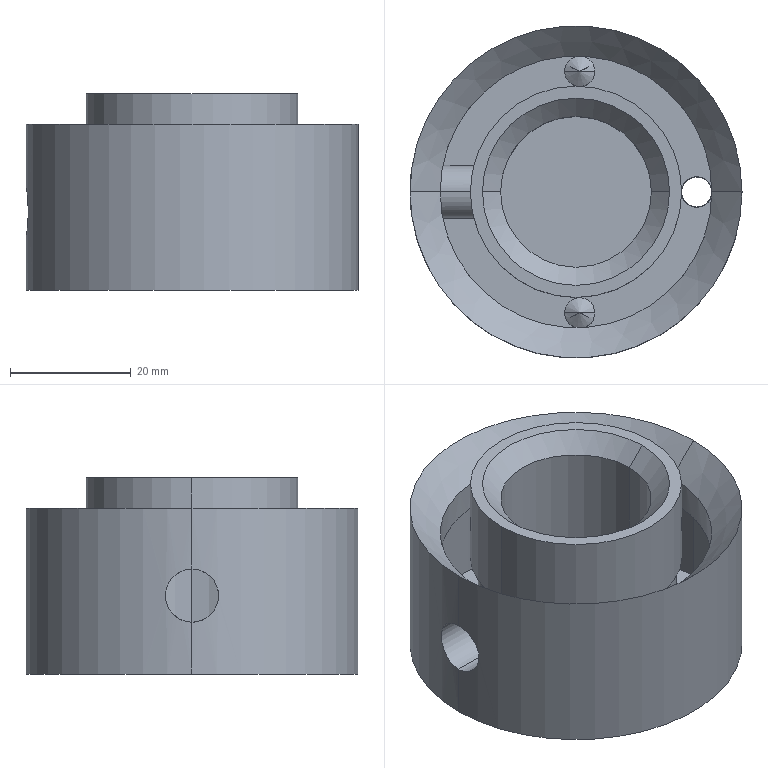Part | 1 solid | 28 faces | box 55 x 55 x 32.5 mm | volume 47312 mm3 | cylinder 16 | cone 8 | plane 4 | commonest cylinder face diameters 5 x6 8.8 x2 25 x2 35 x2 45 x2 55 x2
STEP:
#1=CARTESIAN_POINT('',(-12.5,0.,29.5));
#2=VERTEX_POINT('',#1);
#3=CARTESIAN_POINT('',(12.5,0.,29.5));
#4=VERTEX_POINT('',#3);
#5=CARTESIAN_POINT('',(0.,0.,29.5));
#6=DIRECTION('',(0.,0.,1.));
#7=DIRECTION('',(1.,0.,0.));
#8=AXIS2_PLACEMENT_3D('',#5,#6,#7);
#9=CIRCLE('',#8,12.5);
#10=EDGE_CURVE('',#2,#4,#9,.T.);
#11=ORIENTED_EDGE('',*,*,#10,.F.);
#12=CARTESIAN_POINT('',(-15.5,0.,32.5));
#13=VERTEX_POINT('',#12);
#14=CARTESIAN_POINT('',(-12.5,0.,29.5));
#15=DIRECTION('',(-0.7071,0.,0.7071));
#16=VECTOR('',#15,1000.);
#17=LINE('',#14,#16);
#18=EDGE_CURVE('',#2,#13,#17,.T.);
#19=ORIENTED_EDGE('',*,*,#18,.T.);
#20=CARTESIAN_POINT('',(15.5,0.,32.5));
#21=VERTEX_POINT('',#20);
#22=CARTESIAN_POINT('',(0.,0.,32.5));
#23=DIRECTION('',(0.,0.,-1.));
#24=DIRECTION('',(1.,0.,0.));
#25=AXIS2_PLACEMENT_3D('',#22,#23,#24);
#26=CIRCLE('',#25,15.5);
#27=EDGE_CURVE('',#21,#13,#26,.T.);
#28=ORIENTED_EDGE('',*,*,#27,.F.);
#29=CARTESIAN_POINT('',(12.5,0.,29.5));
#30=DIRECTION('',(0.7071,0.,0.7071));
#31=VECTOR('',#30,1000.);
#32=LINE('',#29,#31);
#33=EDGE_CURVE('',#4,#21,#32,.T.);
#34=ORIENTED_EDGE('',*,*,#33,.F.);
#35=EDGE_LOOP('',(#11,#19,#28,#34));
#36=FACE_OUTER_BOUND('',#35,.T.);
#37=CARTESIAN_POINT('',(0.,0.,29.5));
#38=DIRECTION('',(0.,0.,1.));
#39=DIRECTION('',(1.,0.,0.));
#40=AXIS2_PLACEMENT_3D('',#37,#38,#39);
#41=CONICAL_SURFACE('',#40,12.5,0.7854);
#42=ADVANCED_FACE('',(#36),#41,.F.);
#43=CARTESIAN_POINT('',(17.5,0.,0.));
#44=VERTEX_POINT('',#43);
#45=CARTESIAN_POINT('',(22.5,0.,0.));
#46=VERTEX_POINT('',#45);
#47=CARTESIAN_POINT('',(20.,0.,0.));
#48=DIRECTION('',(0.,0.,1.));
#49=DIRECTION('',(1.,0.,0.));
#50=AXIS2_PLACEMENT_3D('',#47,#48,#49);
#51=CIRCLE('',#50,2.5);
#52=EDGE_CURVE('',#44,#46,#51,.T.);
#53=ORIENTED_EDGE('',*,*,#52,.F.);
#54=CARTESIAN_POINT('',(17.5,0.,17.5));
#55=VERTEX_POINT('',#54);
#56=CARTESIAN_POINT('',(17.5,0.,17.5));
#57=DIRECTION('',(0.,0.,1.));
#58=VECTOR('',#57,1000.);
#59=LINE('',#56,#58);
#60=EDGE_CURVE('',#44,#55,#59,.T.);
#61=ORIENTED_EDGE('',*,*,#60,.T.);
#62=CARTESIAN_POINT('',(22.5,0.,17.5));
#63=VERTEX_POINT('',#62);
#64=CARTESIAN_POINT('',(20.,0.,17.5));
#65=DIRECTION('',(0.,0.,1.));
#66=DIRECTION('',(1.,0.,0.));
#67=AXIS2_PLACEMENT_3D('',#64,#65,#66);
#68=CIRCLE('',#67,2.5);
#69=EDGE_CURVE('',#55,#63,#68,.T.);
#70=ORIENTED_EDGE('',*,*,#69,.T.);
#71=CARTESIAN_POINT('',(22.5,0.,17.5));
#72=DIRECTION('',(0.,0.,1.));
#73=VECTOR('',#72,1000.);
#74=LINE('',#71,#73);
#75=EDGE_CURVE('',#46,#63,#74,.T.);
#76=ORIENTED_EDGE('',*,*,#75,.F.);
#77=EDGE_LOOP('',(#53,#61,#70,#76));
#78=FACE_OUTER_BOUND('',#77,.T.);
#79=CARTESIAN_POINT('',(20.,0.,17.5));
#80=DIRECTION('',(0.,0.,1.));
#81=DIRECTION('',(1.,0.,0.));
#82=AXIS2_PLACEMENT_3D('',#79,#80,#81);
#83=CYLINDRICAL_SURFACE('',#82,2.5);
#84=ADVANCED_FACE('',(#78),#83,.F.);
#85=CARTESIAN_POINT('',(-27.5,0.,17.4));
#86=VERTEX_POINT('',#85);
#87=CARTESIAN_POINT('',(-27.5,0.,8.6));
#88=VERTEX_POINT('',#87);
#89=CARTESIAN_POINT('',(-27.5,0.,17.4));
#90=CARTESIAN_POINT('',(-27.5,-0.2873,17.4));
#91=CARTESIAN_POINT('',(-27.495,-0.5732,17.372));
#92=CARTESIAN_POINT('',(-27.478,-1.142,17.259));
#93=CARTESIAN_POINT('',(-27.465,-1.419,17.175));
#94=CARTESIAN_POINT('',(-27.432,-1.949,16.955));
#95=CARTESIAN_POINT('',(-27.412,-2.205,16.818));
#96=CARTESIAN_POINT('',(-27.37,-2.685,16.498));
#97=CARTESIAN_POINT('',(-27.347,-2.906,16.316));
#98=CARTESIAN_POINT('',(-27.301,-3.312,15.911));
#99=CARTESIAN_POINT('',(-27.277,-3.498,15.685));
#100=CARTESIAN_POINT('',(-27.234,-3.817,15.208));
#101=CARTESIAN_POINT('',(-27.215,-3.952,14.955));
#102=CARTESIAN_POINT('',(-27.182,-4.174,14.422));
#103=CARTESIAN_POINT('',(-27.168,-4.259,14.143));
#104=CARTESIAN_POINT('',(-27.15,-4.371,13.581));
#105=CARTESIAN_POINT('',(-27.146,-4.4,13.293));
#106=CARTESIAN_POINT('',(-27.146,-4.4,12.712));
#107=CARTESIAN_POINT('',(-27.15,-4.372,12.426));
#108=CARTESIAN_POINT('',(-27.168,-4.26,11.863));
#109=CARTESIAN_POINT('',(-27.181,-4.175,11.583));
#110=CARTESIAN_POINT('',(-27.214,-3.955,11.05));
#111=CARTESIAN_POINT('',(-27.234,-3.82,10.798));
#112=CARTESIAN_POINT('',(-27.277,-3.501,10.319));
#113=CARTESIAN_POINT('',(-27.3,-3.316,10.093));
#114=CARTESIAN_POINT('',(-27.346,-2.911,9.688));
#115=CARTESIAN_POINT('',(-27.369,-2.69,9.506));
#116=CARTESIAN_POINT('',(-27.412,-2.209,9.183));
#117=CARTESIAN_POINT('',(-27.432,-1.954,9.047));
#118=CARTESIAN_POINT('',(-27.464,-1.425,8.827));
#119=CARTESIAN_POINT('',(-27.478,-1.147,8.742));
#120=CARTESIAN_POINT('',(-27.495,-0.5788,8.629));
#121=CARTESIAN_POINT('',(-27.5,-0.2911,8.6));
#122=CARTESIAN_POINT('',(-27.5,0.,8.6));
#123=B_SPLINE_CURVE_WITH_KNOTS('',3,(#89,#90,#91,#92,#93,#94,#95,#96,#97,#98,#99,#100,#101,#102,#103,#104,#105,#106,#107,#108,#109,#110,#111,#112,#113,#114,#115,#116,#117,#118,#119,#120,#121,#122),.UNSPECIFIED.,.F.,.F.,(4,2,2,2,2,2,2,2,2,2,2,2,2,2,2,2,4),(0.01378,0.01464,0.0155,0.01636,0.01722,0.01808,0.01894,0.01981,0.02067,0.02153,0.02239,0.02325,0.02411,0.02497,0.02583,0.02669,0.02755),.UNSPECIFIED.);
#124=EDGE_CURVE('',#86,#88,#123,.T.);
#125=ORIENTED_EDGE('',*,*,#124,.F.);
#126=CARTESIAN_POINT('',(-12.5,0.,17.4));
#127=VERTEX_POINT('',#126);
#128=CARTESIAN_POINT('',(0.,0.,17.4));
#129=DIRECTION('',(1.,0.,0.));
#130=VECTOR('',#129,1000.);
#131=LINE('',#128,#130);
#132=EDGE_CURVE('',#86,#127,#131,.T.);
#133=ORIENTED_EDGE('',*,*,#132,.T.);
#134=CARTESIAN_POINT('',(-12.5,0.,8.6));
#135=VERTEX_POINT('',#134);
#136=CARTESIAN_POINT('',(-12.5,0.,17.4));
#137=CARTESIAN_POINT('',(-12.5,-0.2933,17.4));
#138=CARTESIAN_POINT('',(-12.49,-0.5812,17.371));
#139=CARTESIAN_POINT('',(-12.451,-1.147,17.258));
#140=CARTESIAN_POINT('',(-12.421,-1.428,17.172));
#141=CARTESIAN_POINT('',(-12.348,-1.96,16.95));
#142=CARTESIAN_POINT('',(-12.305,-2.211,16.815));
#143=CARTESIAN_POINT('',(-12.21,-2.688,16.495));
#144=CARTESIAN_POINT('',(-12.158,-2.912,16.311));
#145=CARTESIAN_POINT('',(-12.055,-3.314,15.908));
#146=CARTESIAN_POINT('',(-12.003,-3.495,15.688));
#147=CARTESIAN_POINT('',(-11.904,-3.817,15.208));
#148=CARTESIAN_POINT('',(-11.86,-3.952,14.956));
#149=CARTESIAN_POINT('',(-11.803,-4.117,14.56));
#150=CARTESIAN_POINT('',(-11.786,-4.165,14.425));
#151=CARTESIAN_POINT('',(-11.755,-4.25,14.148));
#152=CARTESIAN_POINT('',(-11.742,-4.286,14.006));
#153=CARTESIAN_POINT('',(-11.711,-4.371,13.579));
#154=CARTESIAN_POINT('',(-11.7,-4.4,13.292));
#155=CARTESIAN_POINT('',(-11.7,-4.4,12.713));
#156=CARTESIAN_POINT('',(-11.711,-4.371,12.418));
#157=CARTESIAN_POINT('',(-11.753,-4.257,11.852));
#158=CARTESIAN_POINT('',(-11.783,-4.173,11.577));
#159=CARTESIAN_POINT('',(-11.86,-3.95,11.041));
#160=CARTESIAN_POINT('',(-11.905,-3.814,10.788));
#161=CARTESIAN_POINT('',(-12.002,-3.496,10.314));
#162=CARTESIAN_POINT('',(-12.055,-3.312,10.09));
#163=CARTESIAN_POINT('',(-12.159,-2.908,9.685));
#164=CARTESIAN_POINT('',(-12.21,-2.688,9.505));
#165=CARTESIAN_POINT('',(-12.305,-2.213,9.186));
#166=CARTESIAN_POINT('',(-12.349,-1.955,9.048));
#167=CARTESIAN_POINT('',(-12.421,-1.426,8.828));
#168=CARTESIAN_POINT('',(-12.45,-1.151,8.743));
#169=CARTESIAN_POINT('',(-12.49,-0.5803,8.629));
#170=CARTESIAN_POINT('',(-12.5,-0.2889,8.6));
#171=CARTESIAN_POINT('',(-12.5,0.,8.6));
#172=B_SPLINE_CURVE_WITH_KNOTS('',3,(#136,#137,#138,#139,#140,#141,#142,#143,#144,#145,#146,#147,#148,#149,#150,#151,#152,#153,#154,#155,#156,#157,#158,#159,#160,#161,#162,#163,#164,#165,#166,#167,#168,#169,#170,#171),.UNSPECIFIED.,.F.,.F.,(4,2,2,2,2,2,2,2,2,2,2,2,2,2,2,2,2,4),(0.,0.0008668,0.001734,0.0026,0.003467,0.004334,0.005201,0.005634,0.006067,0.006934,0.007801,0.008668,0.009535,0.0104,0.01127,0.01213,0.013,0.01387),.UNSPECIFIED.);
#173=EDGE_CURVE('',#127,#135,#172,.T.);
#174=ORIENTED_EDGE('',*,*,#173,.T.);
#175=CARTESIAN_POINT('',(0.,0.,8.6));
#176=DIRECTION('',(1.,0.,0.));
#177=VECTOR('',#176,1000.);
#178=LINE('',#175,#177);
#179=EDGE_CURVE('',#88,#135,#178,.T.);
#180=ORIENTED_EDGE('',*,*,#179,.F.);
#181=EDGE_LOOP('',(#125,#133,#174,#180));
#182=FACE_OUTER_BOUND('',#181,.T.);
#183=CARTESIAN_POINT('',(0.,0.,13.));
#184=DIRECTION('',(1.,0.,0.));
#185=DIRECTION('',(0.,0.,-1.));
#186=AXIS2_PLACEMENT_3D('',#183,#184,#185);
#187=CYLINDRICAL_SURFACE('',#186,4.4);
#188=ADVANCED_FACE('',(#182),#187,.F.);
#189=CARTESIAN_POINT('',(3.117,19.99,12.));
#190=VERTEX_POINT('',#189);
#191=CARTESIAN_POINT('',(-1.883,19.99,12.));
#192=VERTEX_POINT('',#191);
#193=CARTESIAN_POINT('',(0.6172,19.99,12.));
#194=DIRECTION('',(0.,0.,-1.));
#195=DIRECTION('',(-1.,0.,0.));
#196=AXIS2_PLACEMENT_3D('',#193,#194,#195);
#197=CIRCLE('',#196,2.5);
#198=EDGE_CURVE('',#190,#192,#197,.T.);
#199=ORIENTED_EDGE('',*,*,#198,.F.);
#200=CARTESIAN_POINT('',(3.117,19.99,0.));
#201=VERTEX_POINT('',#200);
#202=CARTESIAN_POINT('',(3.117,19.99,0.));
#203=DIRECTION('',(0.,0.,-1.));
#204=VECTOR('',#203,1000.);
#205=LINE('',#202,#204);
#206=EDGE_CURVE('',#190,#201,#205,.T.);
#207=ORIENTED_EDGE('',*,*,#206,.T.);
#208=CARTESIAN_POINT('',(-1.883,19.99,0.));
#209=VERTEX_POINT('',#208);
#210=CARTESIAN_POINT('',(0.6172,19.99,0.));
#211=DIRECTION('',(0.,0.,-1.));
#212=DIRECTION('',(-1.,0.,0.));
#213=AXIS2_PLACEMENT_3D('',#210,#211,#212);
#214=CIRCLE('',#213,2.5);
#215=EDGE_CURVE('',#201,#209,#214,.T.);
#216=ORIENTED_EDGE('',*,*,#215,.T.);
#217=CARTESIAN_POINT('',(-1.883,19.99,0.));
#218=DIRECTION('',(0.,0.,-1.));
#219=VECTOR('',#218,1000.);
#220=LINE('',#217,#219);
#221=EDGE_CURVE('',#192,#209,#220,.T.);
#222=ORIENTED_EDGE('',*,*,#221,.F.);
#223=EDGE_LOOP('',(#199,#207,#216,#222));
#224=FACE_OUTER_BOUND('',#223,.T.);
#225=CARTESIAN_POINT('',(0.6172,19.99,0.));
#226=DIRECTION('',(0.,0.,-1.));
#227=DIRECTION('',(-1.,0.,0.));
#228=AXIS2_PLACEMENT_3D('',#225,#226,#227);
#229=CYLINDRICAL_SURFACE('',#228,2.5);
#230=ADVANCED_FACE('',(#224),#229,.F.);
#231=CARTESIAN_POINT('',(0.6172,19.99,13.502));
#232=VERTEX_POINT('',#231);
#233=CARTESIAN_POINT('',(-1.883,19.99,12.));
#234=DIRECTION('',(-0.8572,0.,-0.515));
#235=VECTOR('',#234,1000.);
#236=LINE('',#233,#235);
#237=EDGE_CURVE('',#232,#192,#236,.T.);
#238=ORIENTED_EDGE('',*,*,#237,.F.);
#239=CARTESIAN_POINT('',(3.117,19.99,12.));
#240=DIRECTION('',(0.8572,0.,-0.515));
#241=VECTOR('',#240,1000.);
#242=LINE('',#239,#241);
#243=EDGE_CURVE('',#232,#190,#242,.T.);
#244=ORIENTED_EDGE('',*,*,#243,.T.);
#245=ORIENTED_EDGE('',*,*,#198,.T.);
#246=EDGE_LOOP('',(#238,#244,#245));
#247=FACE_OUTER_BOUND('',#246,.T.);
#248=CARTESIAN_POINT('',(0.6172,19.99,12.));
#249=DIRECTION('',(0.,0.,-1.));
#250=DIRECTION('',(-1.,0.,0.));
#251=AXIS2_PLACEMENT_3D('',#248,#249,#250);
#252=CONICAL_SURFACE('',#251,2.5,1.03);
#253=ADVANCED_FACE('',(#247),#252,.F.);
#254=CARTESIAN_POINT('',(3.12,-20.028,12.));
#255=VERTEX_POINT('',#254);
#256=CARTESIAN_POINT('',(-1.88,-20.028,12.));
#257=VERTEX_POINT('',#256);
#258=CARTESIAN_POINT('',(0.6196,-20.028,12.));
#259=DIRECTION('',(0.,0.,-1.));
#260=DIRECTION('',(-1.,0.,0.));
#261=AXIS2_PLACEMENT_3D('',#258,#259,#260);
#262=CIRCLE('',#261,2.5);
#263=EDGE_CURVE('',#255,#257,#262,.T.);
#264=ORIENTED_EDGE('',*,*,#263,.F.);
#265=CARTESIAN_POINT('',(3.12,-20.028,0.));
#266=VERTEX_POINT('',#265);
#267=CARTESIAN_POINT('',(3.12,-20.028,0.));
#268=DIRECTION('',(0.,0.,-1.));
#269=VECTOR('',#268,1000.);
#270=LINE('',#267,#269);
#271=EDGE_CURVE('',#255,#266,#270,.T.);
#272=ORIENTED_EDGE('',*,*,#271,.T.);
#273=CARTESIAN_POINT('',(-1.88,-20.028,0.));
#274=VERTEX_POINT('',#273);
#275=CARTESIAN_POINT('',(0.6196,-20.028,0.));
#276=DIRECTION('',(0.,0.,-1.));
#277=DIRECTION('',(-1.,0.,0.));
#278=AXIS2_PLACEMENT_3D('',#275,#276,#277);
#279=CIRCLE('',#278,2.5);
#280=EDGE_CURVE('',#266,#274,#279,.T.);
#281=ORIENTED_EDGE('',*,*,#280,.T.);
#282=CARTESIAN_POINT('',(-1.88,-20.028,0.));
#283=DIRECTION('',(0.,0.,-1.));
#284=VECTOR('',#283,1000.);
#285=LINE('',#282,#284);
#286=EDGE_CURVE('',#257,#274,#285,.T.);
#287=ORIENTED_EDGE('',*,*,#286,.F.);
#288=EDGE_LOOP('',(#264,#272,#281,#287));
#289=FACE_OUTER_BOUND('',#288,.T.);
#290=CARTESIAN_POINT('',(0.6196,-20.028,0.));
#291=DIRECTION('',(0.,0.,-1.));
#292=DIRECTION('',(-1.,0.,0.));
#293=AXIS2_PLACEMENT_3D('',#290,#291,#292);
#294=CYLINDRICAL_SURFACE('',#293,2.5);
#295=ADVANCED_FACE('',(#289),#294,.F.);
#296=CARTESIAN_POINT('',(0.6196,-20.028,13.502));
#297=VERTEX_POINT('',#296);
#298=CARTESIAN_POINT('',(-1.88,-20.028,12.));
#299=DIRECTION('',(-0.8572,0.,-0.515));
#300=VECTOR('',#299,1000.);
#301=LINE('',#298,#300);
#302=EDGE_CURVE('',#297,#257,#301,.T.);
#303=ORIENTED_EDGE('',*,*,#302,.F.);
#304=CARTESIAN_POINT('',(3.12,-20.028,12.));
#305=DIRECTION('',(0.8572,0.,-0.515));
#306=VECTOR('',#305,1000.);
#307=LINE('',#304,#306);
#308=EDGE_CURVE('',#297,#255,#307,.T.);
#309=ORIENTED_EDGE('',*,*,#308,.T.);
#310=ORIENTED_EDGE('',*,*,#263,.T.);
#311=EDGE_LOOP('',(#303,#309,#310));
#312=FACE_OUTER_BOUND('',#311,.T.);
#313=CARTESIAN_POINT('',(0.6196,-20.028,12.));
#314=DIRECTION('',(0.,0.,-1.));
#315=DIRECTION('',(-1.,0.,0.));
#316=AXIS2_PLACEMENT_3D('',#313,#314,#315);
#317=CONICAL_SURFACE('',#316,2.5,1.03);
#318=ADVANCED_FACE('',(#312),#317,.F.);
#319=CARTESIAN_POINT('',(-22.5,0.,22.5));
#320=VERTEX_POINT('',#319);
#321=CARTESIAN_POINT('',(22.5,0.,22.5));
#322=VERTEX_POINT('',#321);
#323=CARTESIAN_POINT('',(0.,0.,22.5));
#324=DIRECTION('',(0.,0.,1.));
#325=DIRECTION('',(1.,0.,0.));
#326=AXIS2_PLACEMENT_3D('',#323,#324,#325);
#327=CIRCLE('',#326,22.5);
#328=EDGE_CURVE('',#320,#322,#327,.T.);
#329=ORIENTED_EDGE('',*,*,#328,.F.);
#330=CARTESIAN_POINT('',(-27.5,0.,27.5));
#331=VERTEX_POINT('',#330);
#332=CARTESIAN_POINT('',(-22.5,0.,22.5));
#333=DIRECTION('',(-0.7071,0.,0.7071));
#334=VECTOR('',#333,1000.);
#335=LINE('',#332,#334);
#336=EDGE_CURVE('',#320,#331,#335,.T.);
#337=ORIENTED_EDGE('',*,*,#336,.T.);
#338=CARTESIAN_POINT('',(27.5,0.,27.5));
#339=VERTEX_POINT('',#338);
#340=CARTESIAN_POINT('',(0.,0.,27.5));
#341=DIRECTION('',(0.,0.,1.));
#342=DIRECTION('',(1.,0.,0.));
#343=AXIS2_PLACEMENT_3D('',#340,#341,#342);
#344=CIRCLE('',#343,27.5);
#345=EDGE_CURVE('',#331,#339,#344,.T.);
#346=ORIENTED_EDGE('',*,*,#345,.T.);
#347=CARTESIAN_POINT('',(22.5,0.,22.5));
#348=DIRECTION('',(0.7071,0.,0.7071));
#349=VECTOR('',#348,1000.);
#350=LINE('',#347,#349);
#351=EDGE_CURVE('',#322,#339,#350,.T.);
#352=ORIENTED_EDGE('',*,*,#351,.F.);
#353=EDGE_LOOP('',(#329,#337,#346,#352));
#354=FACE_OUTER_BOUND('',#353,.T.);
#355=CARTESIAN_POINT('',(0.,0.,22.5));
#356=DIRECTION('',(0.,0.,1.));
#357=DIRECTION('',(1.,0.,0.));
#358=AXIS2_PLACEMENT_3D('',#355,#356,#357);
#359=CONICAL_SURFACE('',#358,22.5,0.7854);
#360=ADVANCED_FACE('',(#354),#359,.F.);
#361=CARTESIAN_POINT('',(0.,0.,27.5));
#362=DIRECTION('',(0.,0.,1.));
#363=DIRECTION('',(1.,0.,0.));
#364=AXIS2_PLACEMENT_3D('',#361,#362,#363);
#365=CIRCLE('',#364,27.5);
#366=EDGE_CURVE('',#339,#331,#365,.T.);
#367=ORIENTED_EDGE('',*,*,#366,.F.);
#368=CARTESIAN_POINT('',(27.5,0.,0.));
#369=VERTEX_POINT('',#368);
#370=CARTESIAN_POINT('',(27.5,0.,32.5));
#371=DIRECTION('',(0.,0.,-1.));
#372=VECTOR('',#371,1000.);
#373=LINE('',#370,#372);
#374=EDGE_CURVE('',#339,#369,#373,.T.);
#375=ORIENTED_EDGE('',*,*,#374,.T.);
#376=CARTESIAN_POINT('',(-27.5,0.,0.));
#377=VERTEX_POINT('',#376);
#378=CARTESIAN_POINT('',(0.,0.,0.));
#379=DIRECTION('',(0.,0.,1.));
#380=DIRECTION('',(1.,0.,0.));
#381=AXIS2_PLACEMENT_3D('',#378,#379,#380);
#382=CIRCLE('',#381,27.5);
#383=EDGE_CURVE('',#369,#377,#382,.T.);
#384=ORIENTED_EDGE('',*,*,#383,.T.);
#385=CARTESIAN_POINT('',(-27.5,0.,32.5));
#386=DIRECTION('',(0.,0.,-1.));
#387=VECTOR('',#386,1000.);
#388=LINE('',#385,#387);
#389=EDGE_CURVE('',#88,#377,#388,.T.);
#390=ORIENTED_EDGE('',*,*,#389,.F.);
#391=CARTESIAN_POINT('',(-27.5,0.,8.6));
#392=CARTESIAN_POINT('',(-27.5,0.2912,8.6));
#393=CARTESIAN_POINT('',(-27.495,0.5775,8.629));
#394=CARTESIAN_POINT('',(-27.478,1.141,8.741));
#395=CARTESIAN_POINT('',(-27.465,1.42,8.826));
#396=CARTESIAN_POINT('',(-27.432,1.953,9.047));
#397=CARTESIAN_POINT('',(-27.412,2.205,9.182));
#398=CARTESIAN_POINT('',(-27.37,2.683,9.501));
#399=CARTESIAN_POINT('',(-27.346,2.909,9.687));
#400=CARTESIAN_POINT('',(-27.3,3.315,10.092));
#401=CARTESIAN_POINT('',(-27.277,3.496,10.313));
#402=CARTESIAN_POINT('',(-27.234,3.818,10.794));
#403=CARTESIAN_POINT('',(-27.214,3.955,11.05));
#404=CARTESIAN_POINT('',(-27.182,4.174,11.579));
#405=CARTESIAN_POINT('',(-27.168,4.259,11.857));
#406=CARTESIAN_POINT('',(-27.15,4.372,12.425));
#407=CARTESIAN_POINT('',(-27.146,4.4,12.711));
#408=CARTESIAN_POINT('',(-27.146,4.4,13.286));
#409=CARTESIAN_POINT('',(-27.15,4.371,13.578));
#410=CARTESIAN_POINT('',(-27.168,4.259,14.143));
#411=CARTESIAN_POINT('',(-27.181,4.176,14.417));
#412=CARTESIAN_POINT('',(-27.214,3.955,14.95));
#413=CARTESIAN_POINT('',(-27.234,3.817,15.207));
#414=CARTESIAN_POINT('',(-27.277,3.499,15.684));
#415=CARTESIAN_POINT('',(-27.3,3.316,15.906));
#416=CARTESIAN_POINT('',(-27.347,2.906,16.316));
#417=CARTESIAN_POINT('',(-27.37,2.685,16.498));
#418=CARTESIAN_POINT('',(-27.412,2.209,16.816));
#419=CARTESIAN_POINT('',(-27.432,1.951,16.954));
#420=CARTESIAN_POINT('',(-27.465,1.419,17.175));
#421=CARTESIAN_POINT('',(-27.478,1.144,17.258));
#422=CARTESIAN_POINT('',(-27.495,0.5794,17.371));
#423=CARTESIAN_POINT('',(-27.5,0.2874,17.4));
#424=CARTESIAN_POINT('',(-27.5,0.,17.4));
#425=B_SPLINE_CURVE_WITH_KNOTS('',3,(#391,#392,#393,#394,#395,#396,#397,#398,#399,#400,#401,#402,#403,#404,#405,#406,#407,#408,#409,#410,#411,#412,#413,#414,#415,#416,#417,#418,#419,#420,#421,#422,#423,#424),.UNSPECIFIED.,.F.,.F.,(4,2,2,2,2,2,2,2,2,2,2,2,2,2,2,2,4),(0.,0.0008612,0.001722,0.002583,0.003445,0.004306,0.005167,0.006028,0.006889,0.00775,0.008612,0.009473,0.01033,0.0112,0.01206,0.01292,0.01378),.UNSPECIFIED.);
#426=EDGE_CURVE('',#88,#86,#425,.T.);
#427=ORIENTED_EDGE('',*,*,#426,.T.);
#428=CARTESIAN_POINT('',(-27.5,0.,32.5));
#429=DIRECTION('',(0.,0.,-1.));
#430=VECTOR('',#429,1000.);
#431=LINE('',#428,#430);
#432=EDGE_CURVE('',#331,#86,#431,.T.);
#433=ORIENTED_EDGE('',*,*,#432,.F.);
#434=EDGE_LOOP('',(#367,#375,#384,#390,#427,#433));
#435=FACE_OUTER_BOUND('',#434,.T.);
#436=CARTESIAN_POINT('',(0.,0.,32.5));
#437=DIRECTION('',(0.,0.,-1.));
#438=DIRECTION('',(-1.,0.,0.));
#439=AXIS2_PLACEMENT_3D('',#436,#437,#438);
#440=CYLINDRICAL_SURFACE('',#439,27.5);
#441=ADVANCED_FACE('',(#435),#440,.T.);
#442=ORIENTED_EDGE('',*,*,#10,.T.);
#443=CARTESIAN_POINT('',(12.5,0.,7.));
#444=VERTEX_POINT('',#443);
#445=CARTESIAN_POINT('',(12.5,0.,32.5));
#446=DIRECTION('',(0.,0.,-1.));
#447=VECTOR('',#446,1000.);
#448=LINE('',#445,#447);
#449=EDGE_CURVE('',#4,#444,#448,.T.);
#450=ORIENTED_EDGE('',*,*,#449,.T.);
#451=CARTESIAN_POINT('',(-12.5,0.,7.));
#452=VERTEX_POINT('',#451);
#453=CARTESIAN_POINT('',(0.,0.,7.));
#454=DIRECTION('',(0.,0.,1.));
#455=DIRECTION('',(1.,0.,0.));
#456=AXIS2_PLACEMENT_3D('',#453,#454,#455);
#457=CIRCLE('',#456,12.5);
#458=EDGE_CURVE('',#452,#444,#457,.T.);
#459=ORIENTED_EDGE('',*,*,#458,.F.);
#460=CARTESIAN_POINT('',(-12.5,0.,32.5));
#461=DIRECTION('',(0.,0.,-1.));
#462=VECTOR('',#461,1000.);
#463=LINE('',#460,#462);
#464=EDGE_CURVE('',#135,#452,#463,.T.);
#465=ORIENTED_EDGE('',*,*,#464,.F.);
#466=ORIENTED_EDGE('',*,*,#173,.F.);
#467=CARTESIAN_POINT('',(-12.5,0.,32.5));
#468=DIRECTION('',(0.,0.,-1.));
#469=VECTOR('',#468,1000.);
#470=LINE('',#467,#469);
#471=EDGE_CURVE('',#2,#127,#470,.T.);
#472=ORIENTED_EDGE('',*,*,#471,.F.);
#473=EDGE_LOOP('',(#442,#450,#459,#465,#466,#472));
#474=FACE_OUTER_BOUND('',#473,.T.);
#475=CARTESIAN_POINT('',(0.,0.,32.5));
#476=DIRECTION('',(0.,0.,-1.));
#477=DIRECTION('',(-1.,0.,0.));
#478=AXIS2_PLACEMENT_3D('',#475,#476,#477);
#479=CYLINDRICAL_SURFACE('',#478,12.5);
#480=ADVANCED_FACE('',(#474),#479,.F.);
#481=CARTESIAN_POINT('',(-17.5,0.,17.5));
#482=VERTEX_POINT('',#481);
#483=CARTESIAN_POINT('',(0.,0.,17.5));
#484=DIRECTION('',(0.,0.,-1.));
#485=DIRECTION('',(1.,0.,0.));
#486=AXIS2_PLACEMENT_3D('',#483,#484,#485);
#487=CIRCLE('',#486,17.5);
#488=EDGE_CURVE('',#482,#55,#487,.T.);
#489=ORIENTED_EDGE('',*,*,#488,.F.);
#490=CARTESIAN_POINT('',(-17.5,0.,32.5));
#491=VERTEX_POINT('',#490);
#492=CARTESIAN_POINT('',(-17.5,0.,-63.64));
#493=DIRECTION('',(0.,0.,1.));
#494=VECTOR('',#493,1000.);
#495=LINE('',#492,#494);
#496=EDGE_CURVE('',#482,#491,#495,.T.);
#497=ORIENTED_EDGE('',*,*,#496,.T.);
#498=CARTESIAN_POINT('',(17.5,0.,32.5));
#499=VERTEX_POINT('',#498);
#500=CARTESIAN_POINT('',(0.,0.,32.5));
#501=DIRECTION('',(0.,0.,1.));
#502=DIRECTION('',(1.,0.,0.));
#503=AXIS2_PLACEMENT_3D('',#500,#501,#502);
#504=CIRCLE('',#503,17.5);
#505=EDGE_CURVE('',#499,#491,#504,.T.);
#506=ORIENTED_EDGE('',*,*,#505,.F.);
#507=CARTESIAN_POINT('',(17.5,0.,-63.64));
#508=DIRECTION('',(0.,0.,1.));
#509=VECTOR('',#508,1000.);
#510=LINE('',#507,#509);
#511=EDGE_CURVE('',#55,#499,#510,.T.);
#512=ORIENTED_EDGE('',*,*,#511,.F.);
#513=EDGE_LOOP('',(#489,#497,#506,#512));
#514=FACE_OUTER_BOUND('',#513,.T.);
#515=CARTESIAN_POINT('',(0.,0.,-63.64));
#516=DIRECTION('',(0.,0.,1.));
#517=DIRECTION('',(1.,0.,0.));
#518=AXIS2_PLACEMENT_3D('',#515,#516,#517);
#519=CYLINDRICAL_SURFACE('',#518,17.5);
#520=ADVANCED_FACE('',(#514),#519,.T.);
#521=CARTESIAN_POINT('',(-22.5,0.,17.5));
#522=VERTEX_POINT('',#521);
#523=CARTESIAN_POINT('',(0.,0.,17.5));
#524=DIRECTION('',(0.,0.,-1.));
#525=DIRECTION('',(1.,0.,0.));
#526=AXIS2_PLACEMENT_3D('',#523,#524,#525);
#527=CIRCLE('',#526,22.5);
#528=EDGE_CURVE('',#63,#522,#527,.T.);
#529=ORIENTED_EDGE('',*,*,#528,.T.);
#530=CARTESIAN_POINT('',(-22.5,0.,-63.64));
#531=DIRECTION('',(0.,0.,1.));
#532=VECTOR('',#531,1000.);
#533=LINE('',#530,#532);
#534=EDGE_CURVE('',#522,#320,#533,.T.);
#535=ORIENTED_EDGE('',*,*,#534,.T.);
#536=ORIENTED_EDGE('',*,*,#328,.T.);
#537=CARTESIAN_POINT('',(22.5,0.,-63.64));
#538=DIRECTION('',(0.,0.,1.));
#539=VECTOR('',#538,1000.);
#540=LINE('',#537,#539);
#541=EDGE_CURVE('',#63,#322,#540,.T.);
#542=ORIENTED_EDGE('',*,*,#541,.F.);
#543=EDGE_LOOP('',(#529,#535,#536,#542));
#544=FACE_OUTER_BOUND('',#543,.T.);
#545=CARTESIAN_POINT('',(0.,0.,-63.64));
#546=DIRECTION('',(0.,0.,1.));
#547=DIRECTION('',(1.,0.,0.));
#548=AXIS2_PLACEMENT_3D('',#545,#546,#547);
#549=CYLINDRICAL_SURFACE('',#548,22.5);
#550=ADVANCED_FACE('',(#544),#549,.F.);
#551=ORIENTED_EDGE('',*,*,#534,.F.);
#552=CARTESIAN_POINT('',(0.,0.,17.5));
#553=DIRECTION('',(0.,0.,-1.));
#554=DIRECTION('',(1.,0.,0.));
#555=AXIS2_PLACEMENT_3D('',#552,#553,#554);
#556=CIRCLE('',#555,22.5);
#557=EDGE_CURVE('',#522,#63,#556,.T.);
#558=ORIENTED_EDGE('',*,*,#557,.T.);
#559=ORIENTED_EDGE('',*,*,#541,.T.);
#560=CARTESIAN_POINT('',(0.,0.,22.5));
#561=DIRECTION('',(0.,0.,1.));
#562=DIRECTION('',(1.,0.,0.));
#563=AXIS2_PLACEMENT_3D('',#560,#561,#562);
#564=CIRCLE('',#563,22.5);
#565=EDGE_CURVE('',#322,#320,#564,.T.);
#566=ORIENTED_EDGE('',*,*,#565,.T.);
#567=EDGE_LOOP('',(#551,#558,#559,#566));
#568=FACE_OUTER_BOUND('',#567,.T.);
#569=CARTESIAN_POINT('',(0.,0.,-63.64));
#570=DIRECTION('',(0.,0.,1.));
#571=DIRECTION('',(1.,0.,0.));
#572=AXIS2_PLACEMENT_3D('',#569,#570,#571);
#573=CYLINDRICAL_SURFACE('',#572,22.5);
#574=ADVANCED_FACE('',(#568),#573,.F.);
#575=ORIENTED_EDGE('',*,*,#496,.F.);
#576=CARTESIAN_POINT('',(0.,0.,17.5));
#577=DIRECTION('',(0.,0.,-1.));
#578=DIRECTION('',(1.,0.,0.));
#579=AXIS2_PLACEMENT_3D('',#576,#577,#578);
#580=CIRCLE('',#579,17.5);
#581=EDGE_CURVE('',#55,#482,#580,.T.);
#582=ORIENTED_EDGE('',*,*,#581,.F.);
#583=ORIENTED_EDGE('',*,*,#511,.T.);
#584=CARTESIAN_POINT('',(0.,0.,32.5));
#585=DIRECTION('',(0.,0.,1.));
#586=DIRECTION('',(1.,0.,0.));
#587=AXIS2_PLACEMENT_3D('',#584,#585,#586);
#588=CIRCLE('',#587,17.5);
#589=EDGE_CURVE('',#491,#499,#588,.T.);
#590=ORIENTED_EDGE('',*,*,#589,.F.);
#591=EDGE_LOOP('',(#575,#582,#583,#590));
#592=FACE_OUTER_BOUND('',#591,.T.);
#593=CARTESIAN_POINT('',(0.,0.,-63.64));
#594=DIRECTION('',(0.,0.,1.));
#595=DIRECTION('',(1.,0.,0.));
#596=AXIS2_PLACEMENT_3D('',#593,#594,#595);
#597=CYLINDRICAL_SURFACE('',#596,17.5);
#598=ADVANCED_FACE('',(#592),#597,.T.);
#599=CARTESIAN_POINT('',(20.,0.,17.5));
#600=DIRECTION('',(0.,0.,1.));
#601=DIRECTION('',(1.,0.,0.));
#602=AXIS2_PLACEMENT_3D('',#599,#600,#601);
#603=CIRCLE('',#602,2.5);
#604=EDGE_CURVE('',#63,#55,#603,.T.);
#605=ORIENTED_EDGE('',*,*,#604,.F.);
#606=ORIENTED_EDGE('',*,*,#557,.F.);
#607=ORIENTED_EDGE('',*,*,#528,.F.);
#608=ORIENTED_EDGE('',*,*,#69,.F.);
#609=ORIENTED_EDGE('',*,*,#581,.T.);
#610=ORIENTED_EDGE('',*,*,#488,.T.);
#611=EDGE_LOOP('',(#605,#606,#607,#608,#609,#610));
#612=FACE_OUTER_BOUND('',#611,.T.);
#613=CARTESIAN_POINT('',(0.,0.,17.5));
#614=DIRECTION('',(0.,0.,1.));
#615=DIRECTION('',(1.,0.,0.));
#616=AXIS2_PLACEMENT_3D('',#613,#614,#615);
#617=PLANE('',#616);
#618=ADVANCED_FACE('',(#612),#617,.T.);
#619=ORIENTED_EDGE('',*,*,#449,.F.);
#620=CARTESIAN_POINT('',(0.,0.,29.5));
#621=DIRECTION('',(0.,0.,1.));
#622=DIRECTION('',(1.,0.,0.));
#623=AXIS2_PLACEMENT_3D('',#620,#621,#622);
#624=CIRCLE('',#623,12.5);
#625=EDGE_CURVE('',#4,#2,#624,.T.);
#626=ORIENTED_EDGE('',*,*,#625,.T.);
#627=ORIENTED_EDGE('',*,*,#471,.T.);
#628=CARTESIAN_POINT('',(-12.5,0.,8.6));
#629=CARTESIAN_POINT('',(-12.5,0.2888,8.6));
#630=CARTESIAN_POINT('',(-12.49,0.5802,8.629));
#631=CARTESIAN_POINT('',(-12.45,1.151,8.743));
#632=CARTESIAN_POINT('',(-12.421,1.426,8.828));
#633=CARTESIAN_POINT('',(-12.349,1.957,9.049));
#634=CARTESIAN_POINT('',(-12.305,2.215,9.187));
#635=CARTESIAN_POINT('',(-12.21,2.689,9.506));
#636=CARTESIAN_POINT('',(-12.159,2.909,9.687));
#637=CARTESIAN_POINT('',(-12.054,3.316,10.093));
#638=CARTESIAN_POINT('',(-12.002,3.498,10.315));
#639=CARTESIAN_POINT('',(-11.905,3.814,10.788));
#640=CARTESIAN_POINT('',(-11.86,3.952,11.043));
#641=CARTESIAN_POINT('',(-11.783,4.174,11.577));
#642=CARTESIAN_POINT('',(-11.753,4.257,11.852));
#643=CARTESIAN_POINT('',(-11.711,4.371,12.417));
#644=CARTESIAN_POINT('',(-11.7,4.4,12.711));
#645=CARTESIAN_POINT('',(-11.7,4.4,13.291));
#646=CARTESIAN_POINT('',(-11.711,4.371,13.578));
#647=CARTESIAN_POINT('',(-11.753,4.257,14.148));
#648=CARTESIAN_POINT('',(-11.784,4.172,14.428));
#649=CARTESIAN_POINT('',(-11.86,3.951,14.957));
#650=CARTESIAN_POINT('',(-11.905,3.814,15.212));
#651=CARTESIAN_POINT('',(-12.003,3.494,15.69));
#652=CARTESIAN_POINT('',(-12.055,3.313,15.91));
#653=CARTESIAN_POINT('',(-12.158,2.91,16.313));
#654=CARTESIAN_POINT('',(-12.211,2.685,16.498));
#655=CARTESIAN_POINT('',(-12.305,2.21,16.815));
#656=CARTESIAN_POINT('',(-12.349,1.959,16.951));
#657=CARTESIAN_POINT('',(-12.421,1.426,17.173));
#658=CARTESIAN_POINT('',(-12.451,1.146,17.258));
#659=CARTESIAN_POINT('',(-12.49,0.581,17.371));
#660=CARTESIAN_POINT('',(-12.5,0.2932,17.4));
#661=CARTESIAN_POINT('',(-12.5,0.,17.4));
#662=B_SPLINE_CURVE_WITH_KNOTS('',3,(#628,#629,#630,#631,#632,#633,#634,#635,#636,#637,#638,#639,#640,#641,#642,#643,#644,#645,#646,#647,#648,#649,#650,#651,#652,#653,#654,#655,#656,#657,#658,#659,#660,#661),.UNSPECIFIED.,.F.,.F.,(4,2,2,2,2,2,2,2,2,2,2,2,2,2,2,2,4),(0.01387,0.01474,0.0156,0.01647,0.01733,0.0182,0.01907,0.01993,0.0208,0.02167,0.02253,0.0234,0.02427,0.02513,0.026,0.02687,0.02773),.UNSPECIFIED.);
#663=EDGE_CURVE('',#135,#127,#662,.T.);
#664=ORIENTED_EDGE('',*,*,#663,.F.);
#665=ORIENTED_EDGE('',*,*,#464,.T.);
#666=CARTESIAN_POINT('',(0.,0.,7.));
#667=DIRECTION('',(0.,0.,1.));
#668=DIRECTION('',(1.,0.,0.));
#669=AXIS2_PLACEMENT_3D('',#666,#667,#668);
#670=CIRCLE('',#669,12.5);
#671=EDGE_CURVE('',#444,#452,#670,.T.);
#672=ORIENTED_EDGE('',*,*,#671,.F.);
#673=EDGE_LOOP('',(#619,#626,#627,#664,#665,#672));
#674=FACE_OUTER_BOUND('',#673,.T.);
#675=CARTESIAN_POINT('',(0.,0.,32.5));
#676=DIRECTION('',(0.,0.,-1.));
#677=DIRECTION('',(-1.,0.,0.));
#678=AXIS2_PLACEMENT_3D('',#675,#676,#677);
#679=CYLINDRICAL_SURFACE('',#678,12.5);
#680=ADVANCED_FACE('',(#674),#679,.F.);
#681=ORIENTED_EDGE('',*,*,#27,.T.);
#682=CARTESIAN_POINT('',(0.,0.,32.5));
#683=DIRECTION('',(0.,0.,-1.));
#684=DIRECTION('',(1.,0.,0.));
#685=AXIS2_PLACEMENT_3D('',#682,#683,#684);
#686=CIRCLE('',#685,15.5);
#687=EDGE_CURVE('',#13,#21,#686,.T.);
#688=ORIENTED_EDGE('',*,*,#687,.T.);
#689=EDGE_LOOP('',(#681,#688));
#690=FACE_BOUND('',#689,.T.);
#691=ORIENTED_EDGE('',*,*,#505,.T.);
#692=ORIENTED_EDGE('',*,*,#589,.T.);
#693=EDGE_LOOP('',(#691,#692));
#694=FACE_OUTER_BOUND('',#693,.T.);
#695=CARTESIAN_POINT('',(0.,0.,32.5));
#696=DIRECTION('',(0.,0.,1.));
#697=DIRECTION('',(1.,0.,0.));
#698=AXIS2_PLACEMENT_3D('',#695,#696,#697);
#699=PLANE('',#698);
#700=ADVANCED_FACE('',(#690,#694),#699,.T.);
#701=CARTESIAN_POINT('',(20.,0.,0.));
#702=DIRECTION('',(0.,0.,1.));
#703=DIRECTION('',(1.,0.,0.));
#704=AXIS2_PLACEMENT_3D('',#701,#702,#703);
#705=CIRCLE('',#704,2.5);
#706=EDGE_CURVE('',#46,#44,#705,.T.);
#707=ORIENTED_EDGE('',*,*,#706,.T.);
#708=ORIENTED_EDGE('',*,*,#52,.T.);
#709=EDGE_LOOP('',(#707,#708));
#710=FACE_BOUND('',#709,.T.);
#711=CARTESIAN_POINT('',(0.6172,19.99,0.));
#712=DIRECTION('',(0.,0.,-1.));
#713=DIRECTION('',(-1.,0.,0.));
#714=AXIS2_PLACEMENT_3D('',#711,#712,#713);
#715=CIRCLE('',#714,2.5);
#716=EDGE_CURVE('',#209,#201,#715,.T.);
#717=ORIENTED_EDGE('',*,*,#716,.F.);
#718=ORIENTED_EDGE('',*,*,#215,.F.);
#719=EDGE_LOOP('',(#717,#718));
#720=FACE_BOUND('',#719,.T.);
#721=CARTESIAN_POINT('',(0.6196,-20.028,0.));
#722=DIRECTION('',(0.,0.,-1.));
#723=DIRECTION('',(-1.,0.,0.));
#724=AXIS2_PLACEMENT_3D('',#721,#722,#723);
#725=CIRCLE('',#724,2.5);
#726=EDGE_CURVE('',#274,#266,#725,.T.);
#727=ORIENTED_EDGE('',*,*,#726,.F.);
#728=ORIENTED_EDGE('',*,*,#280,.F.);
#729=EDGE_LOOP('',(#727,#728));
#730=FACE_BOUND('',#729,.T.);
#731=CARTESIAN_POINT('',(0.,0.,0.));
#732=DIRECTION('',(0.,0.,1.));
#733=DIRECTION('',(1.,0.,0.));
#734=AXIS2_PLACEMENT_3D('',#731,#732,#733);
#735=CIRCLE('',#734,27.5);
#736=EDGE_CURVE('',#377,#369,#735,.T.);
#737=ORIENTED_EDGE('',*,*,#736,.F.);
#738=ORIENTED_EDGE('',*,*,#383,.F.);
#739=EDGE_LOOP('',(#737,#738));
#740=FACE_OUTER_BOUND('',#739,.T.);
#741=CARTESIAN_POINT('',(0.,0.,0.));
#742=DIRECTION('',(0.,0.,1.));
#743=DIRECTION('',(1.,0.,0.));
#744=AXIS2_PLACEMENT_3D('',#741,#742,#743);
#745=PLANE('',#744);
#746=ADVANCED_FACE('',(#710,#720,#730,#740),#745,.F.);
#747=ORIENTED_EDGE('',*,*,#374,.F.);
#748=ORIENTED_EDGE('',*,*,#345,.F.);
#749=ORIENTED_EDGE('',*,*,#432,.T.);
#750=ORIENTED_EDGE('',*,*,#124,.T.);
#751=ORIENTED_EDGE('',*,*,#389,.T.);
#752=ORIENTED_EDGE('',*,*,#736,.T.);
#753=EDGE_LOOP('',(#747,#748,#749,#750,#751,#752));
#754=FACE_OUTER_BOUND('',#753,.T.);
#755=CARTESIAN_POINT('',(0.,0.,32.5));
#756=DIRECTION('',(0.,0.,-1.));
#757=DIRECTION('',(-1.,0.,0.));
#758=AXIS2_PLACEMENT_3D('',#755,#756,#757);
#759=CYLINDRICAL_SURFACE('',#758,27.5);
#760=ADVANCED_FACE('',(#754),#759,.T.);
#761=ORIENTED_EDGE('',*,*,#336,.F.);
#762=ORIENTED_EDGE('',*,*,#565,.F.);
#763=ORIENTED_EDGE('',*,*,#351,.T.);
#764=ORIENTED_EDGE('',*,*,#366,.T.);
#765=EDGE_LOOP('',(#761,#762,#763,#764));
#766=FACE_OUTER_BOUND('',#765,.T.);
#767=CARTESIAN_POINT('',(0.,0.,22.5));
#768=DIRECTION('',(0.,0.,1.));
#769=DIRECTION('',(1.,0.,0.));
#770=AXIS2_PLACEMENT_3D('',#767,#768,#769);
#771=CONICAL_SURFACE('',#770,22.5,0.7854);
#772=ADVANCED_FACE('',(#766),#771,.F.);
#773=ORIENTED_EDGE('',*,*,#308,.F.);
#774=ORIENTED_EDGE('',*,*,#302,.T.);
#775=CARTESIAN_POINT('',(0.6196,-20.028,12.));
#776=DIRECTION('',(0.,0.,-1.));
#777=DIRECTION('',(-1.,0.,0.));
#778=AXIS2_PLACEMENT_3D('',#775,#776,#777);
#779=CIRCLE('',#778,2.5);
#780=EDGE_CURVE('',#257,#255,#779,.T.);
#781=ORIENTED_EDGE('',*,*,#780,.T.);
#782=EDGE_LOOP('',(#773,#774,#781));
#783=FACE_OUTER_BOUND('',#782,.T.);
#784=CARTESIAN_POINT('',(0.6196,-20.028,12.));
#785=DIRECTION('',(0.,0.,-1.));
#786=DIRECTION('',(-1.,0.,0.));
#787=AXIS2_PLACEMENT_3D('',#784,#785,#786);
#788=CONICAL_SURFACE('',#787,2.5,1.03);
#789=ADVANCED_FACE('',(#783),#788,.F.);
#790=ORIENTED_EDGE('',*,*,#271,.F.);
#791=ORIENTED_EDGE('',*,*,#780,.F.);
#792=ORIENTED_EDGE('',*,*,#286,.T.);
#793=ORIENTED_EDGE('',*,*,#726,.T.);
#794=EDGE_LOOP('',(#790,#791,#792,#793));
#795=FACE_OUTER_BOUND('',#794,.T.);
#796=CARTESIAN_POINT('',(0.6196,-20.028,0.));
#797=DIRECTION('',(0.,0.,-1.));
#798=DIRECTION('',(-1.,0.,0.));
#799=AXIS2_PLACEMENT_3D('',#796,#797,#798);
#800=CYLINDRICAL_SURFACE('',#799,2.5);
#801=ADVANCED_FACE('',(#795),#800,.F.);
#802=ORIENTED_EDGE('',*,*,#243,.F.);
#803=ORIENTED_EDGE('',*,*,#237,.T.);
#804=CARTESIAN_POINT('',(0.6172,19.99,12.));
#805=DIRECTION('',(0.,0.,-1.));
#806=DIRECTION('',(-1.,0.,0.));
#807=AXIS2_PLACEMENT_3D('',#804,#805,#806);
#808=CIRCLE('',#807,2.5);
#809=EDGE_CURVE('',#192,#190,#808,.T.);
#810=ORIENTED_EDGE('',*,*,#809,.T.);
#811=EDGE_LOOP('',(#802,#803,#810));
#812=FACE_OUTER_BOUND('',#811,.T.);
#813=CARTESIAN_POINT('',(0.6172,19.99,12.));
#814=DIRECTION('',(0.,0.,-1.));
#815=DIRECTION('',(-1.,0.,0.));
#816=AXIS2_PLACEMENT_3D('',#813,#814,#815);
#817=CONICAL_SURFACE('',#816,2.5,1.03);
#818=ADVANCED_FACE('',(#812),#817,.F.);
#819=ORIENTED_EDGE('',*,*,#206,.F.);
#820=ORIENTED_EDGE('',*,*,#809,.F.);
#821=ORIENTED_EDGE('',*,*,#221,.T.);
#822=ORIENTED_EDGE('',*,*,#716,.T.);
#823=EDGE_LOOP('',(#819,#820,#821,#822));
#824=FACE_OUTER_BOUND('',#823,.T.);
#825=CARTESIAN_POINT('',(0.6172,19.99,0.));
#826=DIRECTION('',(0.,0.,-1.));
#827=DIRECTION('',(-1.,0.,0.));
#828=AXIS2_PLACEMENT_3D('',#825,#826,#827);
#829=CYLINDRICAL_SURFACE('',#828,2.5);
#830=ADVANCED_FACE('',(#824),#829,.F.);
#831=ORIENTED_EDGE('',*,*,#458,.T.);
#832=ORIENTED_EDGE('',*,*,#671,.T.);
#833=EDGE_LOOP('',(#831,#832));
#834=FACE_OUTER_BOUND('',#833,.T.);
#835=CARTESIAN_POINT('',(0.,0.,7.));
#836=DIRECTION('',(0.,0.,1.));
#837=DIRECTION('',(1.,0.,0.));
#838=AXIS2_PLACEMENT_3D('',#835,#836,#837);
#839=PLANE('',#838);
#840=ADVANCED_FACE('',(#834),#839,.T.);
#841=ORIENTED_EDGE('',*,*,#132,.F.);
#842=ORIENTED_EDGE('',*,*,#426,.F.);
#843=ORIENTED_EDGE('',*,*,#179,.T.);
#844=ORIENTED_EDGE('',*,*,#663,.T.);
#845=EDGE_LOOP('',(#841,#842,#843,#844));
#846=FACE_OUTER_BOUND('',#845,.T.);
#847=CARTESIAN_POINT('',(0.,0.,13.));
#848=DIRECTION('',(1.,0.,0.));
#849=DIRECTION('',(0.,0.,-1.));
#850=AXIS2_PLACEMENT_3D('',#847,#848,#849);
#851=CYLINDRICAL_SURFACE('',#850,4.4);
#852=ADVANCED_FACE('',(#846),#851,.F.);
#853=ORIENTED_EDGE('',*,*,#60,.F.);
#854=ORIENTED_EDGE('',*,*,#706,.F.);
#855=ORIENTED_EDGE('',*,*,#75,.T.);
#856=ORIENTED_EDGE('',*,*,#604,.T.);
#857=EDGE_LOOP('',(#853,#854,#855,#856));
#858=FACE_OUTER_BOUND('',#857,.T.);
#859=CARTESIAN_POINT('',(20.,0.,17.5));
#860=DIRECTION('',(0.,0.,1.));
#861=DIRECTION('',(1.,0.,0.));
#862=AXIS2_PLACEMENT_3D('',#859,#860,#861);
#863=CYLINDRICAL_SURFACE('',#862,2.5);
#864=ADVANCED_FACE('',(#858),#863,.F.);
#865=ORIENTED_EDGE('',*,*,#18,.F.);
#866=ORIENTED_EDGE('',*,*,#625,.F.);
#867=ORIENTED_EDGE('',*,*,#33,.T.);
#868=ORIENTED_EDGE('',*,*,#687,.F.);
#869=EDGE_LOOP('',(#865,#866,#867,#868));
#870=FACE_OUTER_BOUND('',#869,.T.);
#871=CARTESIAN_POINT('',(0.,0.,29.5));
#872=DIRECTION('',(0.,0.,1.));
#873=DIRECTION('',(1.,0.,0.));
#874=AXIS2_PLACEMENT_3D('',#871,#872,#873);
#875=CONICAL_SURFACE('',#874,12.5,0.7854);
#876=ADVANCED_FACE('',(#870),#875,.F.);
#877=CLOSED_SHELL('',(#42,#84,#188,#230,#253,#295,#318,#360,#441,#480,#520,#550,#574,#598,#618,#680,#700,#746,#760,#772,#789,#801,#818,#830,#840,#852,#864,#876));
#878=MANIFOLD_SOLID_BREP('',#877);
#879=CARTESIAN_POINT('',(0.,0.,0.));
#880=DIRECTION('',(0.,0.,1.));
#881=DIRECTION('',(1.,0.,0.));
#882=AXIS2_PLACEMENT_3D('',#879,#880,#881);
#883=(LENGTH_UNIT()NAMED_UNIT(*)SI_UNIT(.MILLI.,.METRE.));
#884=UNCERTAINTY_MEASURE_WITH_UNIT(LENGTH_MEASURE(0.00001),#883,'','');
#885=(NAMED_UNIT(*)PLANE_ANGLE_UNIT()SI_UNIT($,.RADIAN.));
#886=(NAMED_UNIT(*)SI_UNIT($,.STERADIAN.)SOLID_ANGLE_UNIT());
#887=(GEOMETRIC_REPRESENTATION_CONTEXT(3)GLOBAL_UNCERTAINTY_ASSIGNED_CONTEXT((#884))GLOBAL_UNIT_ASSIGNED_CONTEXT((#883,#885,#886))REPRESENTATION_CONTEXT('',''));
#888=ADVANCED_BREP_SHAPE_REPRESENTATION('',(#878,#882),#887);